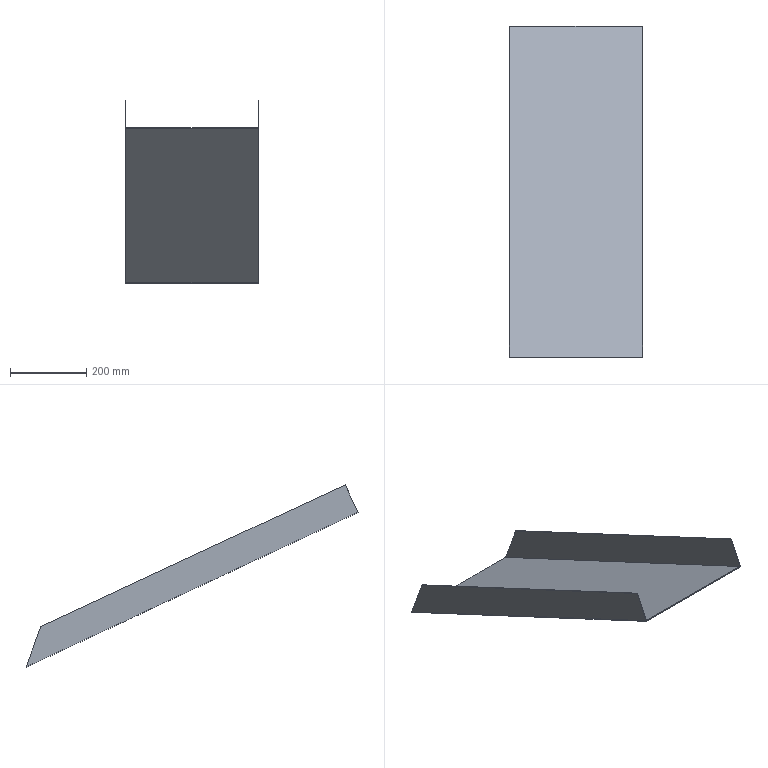Part | NX | features solid 2 | 1 solid | 10 faces | box 350 x 870.242 x 478.305 mm | volume 958236 mm3 | plane 10
STEP:
#1=CARTESIAN_POINT('',(20.,289.829,-157.495));
#2=VERTEX_POINT('',#1);
#3=CARTESIAN_POINT('',(22.,289.829,-157.495));
#4=VERTEX_POINT('',#3);
#5=CARTESIAN_POINT('',(1210.,289.829,-157.495));
#6=DIRECTION('',(-1.,0.,0.));
#7=VECTOR('',#6,1000.);
#8=LINE('',#5,#7);
#9=EDGE_CURVE('',#2,#4,#8,.F.);
#10=ORIENTED_EDGE('',*,*,#9,.F.);
#11=CARTESIAN_POINT('',(20.,256.02,-230.));
#12=VERTEX_POINT('',#11);
#13=CARTESIAN_POINT('',(20.,289.829,-157.495));
#14=DIRECTION('',(0.,-0.4226,-0.9063));
#15=VECTOR('',#14,1000.);
#16=LINE('',#13,#15);
#17=EDGE_CURVE('',#2,#12,#16,.T.);
#18=ORIENTED_EDGE('',*,*,#17,.T.);
#19=CARTESIAN_POINT('',(370.,256.02,-230.));
#20=VERTEX_POINT('',#19);
#21=CARTESIAN_POINT('',(1210.,256.02,-230.));
#22=DIRECTION('',(-1.,0.,0.));
#23=VECTOR('',#22,1000.);
#24=LINE('',#21,#23);
#25=EDGE_CURVE('',#12,#20,#24,.F.);
#26=ORIENTED_EDGE('',*,*,#25,.T.);
#27=CARTESIAN_POINT('',(370.,289.829,-157.495));
#28=VERTEX_POINT('',#27);
#29=CARTESIAN_POINT('',(370.,289.829,-157.495));
#30=DIRECTION('',(0.,-0.4226,-0.9063));
#31=VECTOR('',#30,1000.);
#32=LINE('',#29,#31);
#33=EDGE_CURVE('',#28,#20,#32,.T.);
#34=ORIENTED_EDGE('',*,*,#33,.F.);
#35=CARTESIAN_POINT('',(368.,289.829,-157.495));
#36=VERTEX_POINT('',#35);
#37=CARTESIAN_POINT('',(1210.,289.829,-157.495));
#38=DIRECTION('',(-1.,0.,0.));
#39=VECTOR('',#38,1000.);
#40=LINE('',#37,#39);
#41=EDGE_CURVE('',#36,#28,#40,.F.);
#42=ORIENTED_EDGE('',*,*,#41,.F.);
#43=CARTESIAN_POINT('',(368.,256.865,-228.187));
#44=VERTEX_POINT('',#43);
#45=CARTESIAN_POINT('',(368.,289.829,-157.495));
#46=DIRECTION('',(0.,-0.4226,-0.9063));
#47=VECTOR('',#46,1000.);
#48=LINE('',#45,#47);
#49=EDGE_CURVE('',#36,#44,#48,.T.);
#50=ORIENTED_EDGE('',*,*,#49,.T.);
#51=CARTESIAN_POINT('',(22.,256.865,-228.187));
#52=VERTEX_POINT('',#51);
#53=CARTESIAN_POINT('',(10.,256.865,-228.187));
#54=DIRECTION('',(-1.,0.,0.));
#55=VECTOR('',#54,1000.);
#56=LINE('',#53,#55);
#57=EDGE_CURVE('',#52,#44,#56,.F.);
#58=ORIENTED_EDGE('',*,*,#57,.F.);
#59=CARTESIAN_POINT('',(22.,289.829,-157.495));
#60=DIRECTION('',(0.,-0.4226,-0.9063));
#61=VECTOR('',#60,1000.);
#62=LINE('',#59,#61);
#63=EDGE_CURVE('',#4,#52,#62,.T.);
#64=ORIENTED_EDGE('',*,*,#63,.F.);
#65=EDGE_LOOP('',(#10,#18,#26,#34,#42,#50,#58,#64));
#66=FACE_BOUND('',#65,.T.);
#67=CARTESIAN_POINT('',(1210.,289.829,-157.495));
#68=DIRECTION('',(0.,-0.9063,0.4226));
#69=DIRECTION('',(0.,-0.4226,-0.9063));
#70=AXIS2_PLACEMENT_3D('',#67,#68,#69);
#71=PLANE('',#70);
#72=ADVANCED_FACE('',(#66),#71,.T.);
#73=CARTESIAN_POINT('',(368.,1087.566,-529.486));
#74=VERTEX_POINT('',#73);
#75=CARTESIAN_POINT('',(368.,-205.417,73.442));
#76=DIRECTION('',(0.,-0.9063,0.4226));
#77=VECTOR('',#76,1000.);
#78=LINE('',#75,#77);
#79=EDGE_CURVE('',#36,#74,#78,.F.);
#80=ORIENTED_EDGE('',*,*,#79,.F.);
#81=ORIENTED_EDGE('',*,*,#41,.T.);
#82=CARTESIAN_POINT('',(370.,1087.566,-529.486));
#83=VERTEX_POINT('',#82);
#84=CARTESIAN_POINT('',(370.,-205.417,73.442));
#85=DIRECTION('',(0.,0.9063,-0.4226));
#86=VECTOR('',#85,1000.);
#87=LINE('',#84,#86);
#88=EDGE_CURVE('',#28,#83,#87,.T.);
#89=ORIENTED_EDGE('',*,*,#88,.T.);
#90=CARTESIAN_POINT('',(10.,1087.566,-529.486));
#91=DIRECTION('',(1.,0.,0.));
#92=VECTOR('',#91,1000.);
#93=LINE('',#90,#92);
#94=EDGE_CURVE('',#74,#83,#93,.T.);
#95=ORIENTED_EDGE('',*,*,#94,.F.);
#96=EDGE_LOOP('',(#80,#81,#89,#95));
#97=FACE_BOUND('',#96,.T.);
#98=CARTESIAN_POINT('',(10.,-205.417,73.442));
#99=DIRECTION('',(0.,0.4226,0.9063));
#100=DIRECTION('',(0.,0.9063,-0.4226));
#101=AXIS2_PLACEMENT_3D('',#98,#99,#100);
#102=PLANE('',#101);
#103=ADVANCED_FACE('',(#97),#102,.T.);
#104=ORIENTED_EDGE('',*,*,#88,.F.);
#105=ORIENTED_EDGE('',*,*,#33,.T.);
#106=CARTESIAN_POINT('',(370.,1126.262,-635.8));
#107=VERTEX_POINT('',#106);
#108=CARTESIAN_POINT('',(370.,-239.226,0.9369));
#109=DIRECTION('',(0.,0.9063,-0.4226));
#110=VECTOR('',#109,1000.);
#111=LINE('',#108,#110);
#112=EDGE_CURVE('',#20,#107,#111,.T.);
#113=ORIENTED_EDGE('',*,*,#112,.T.);
#114=CARTESIAN_POINT('',(370.,742.539,418.469));
#115=DIRECTION('',(0.,-0.342,0.9397));
#116=VECTOR('',#115,1000.);
#117=LINE('',#114,#116);
#118=EDGE_CURVE('',#83,#107,#117,.F.);
#119=ORIENTED_EDGE('',*,*,#118,.F.);
#120=EDGE_LOOP('',(#104,#105,#113,#119));
#121=FACE_BOUND('',#120,.T.);
#122=CARTESIAN_POINT('',(370.,-205.417,73.442));
#123=DIRECTION('',(1.,0.,0.));
#124=DIRECTION('',(0.,0.,1.));
#125=AXIS2_PLACEMENT_3D('',#122,#123,#124);
#126=PLANE('',#125);
#127=ADVANCED_FACE('',(#121),#126,.T.);
#128=CARTESIAN_POINT('',(20.,1126.262,-635.8));
#129=VERTEX_POINT('',#128);
#130=CARTESIAN_POINT('',(20.,701.624,-437.789));
#131=DIRECTION('',(0.,-0.9063,0.4226));
#132=VECTOR('',#131,1000.);
#133=LINE('',#130,#132);
#134=EDGE_CURVE('',#129,#12,#133,.T.);
#135=ORIENTED_EDGE('',*,*,#134,.T.);
#136=ORIENTED_EDGE('',*,*,#17,.F.);
#137=CARTESIAN_POINT('',(20.,1087.566,-529.486));
#138=VERTEX_POINT('',#137);
#139=CARTESIAN_POINT('',(20.,735.434,-365.284));
#140=DIRECTION('',(0.,-0.9063,0.4226));
#141=VECTOR('',#140,1000.);
#142=LINE('',#139,#141);
#143=EDGE_CURVE('',#138,#2,#142,.T.);
#144=ORIENTED_EDGE('',*,*,#143,.F.);
#145=CARTESIAN_POINT('',(20.,993.601,-271.319));
#146=DIRECTION('',(0.,0.342,-0.9397));
#147=VECTOR('',#146,1000.);
#148=LINE('',#145,#147);
#149=EDGE_CURVE('',#129,#138,#148,.F.);
#150=ORIENTED_EDGE('',*,*,#149,.F.);
#151=EDGE_LOOP('',(#135,#136,#144,#150));
#152=FACE_BOUND('',#151,.T.);
#153=CARTESIAN_POINT('',(20.,735.434,-365.284));
#154=DIRECTION('',(-1.,0.,0.));
#155=DIRECTION('',(0.,0.,-1.));
#156=AXIS2_PLACEMENT_3D('',#153,#154,#155);
#157=PLANE('',#156);
#158=ADVANCED_FACE('',(#152),#157,.T.);
#159=ORIENTED_EDGE('',*,*,#143,.T.);
#160=ORIENTED_EDGE('',*,*,#9,.T.);
#161=CARTESIAN_POINT('',(22.,1087.566,-529.486));
#162=VERTEX_POINT('',#161);
#163=CARTESIAN_POINT('',(22.,-205.417,73.442));
#164=DIRECTION('',(0.,0.9063,-0.4226));
#165=VECTOR('',#164,1000.);
#166=LINE('',#163,#165);
#167=EDGE_CURVE('',#162,#4,#166,.F.);
#168=ORIENTED_EDGE('',*,*,#167,.F.);
#169=CARTESIAN_POINT('',(22.,1087.566,-529.486));
#170=DIRECTION('',(-1.,0.,0.));
#171=VECTOR('',#170,1000.);
#172=LINE('',#169,#171);
#173=EDGE_CURVE('',#138,#162,#172,.F.);
#174=ORIENTED_EDGE('',*,*,#173,.F.);
#175=EDGE_LOOP('',(#159,#160,#168,#174));
#176=FACE_BOUND('',#175,.T.);
#177=CARTESIAN_POINT('',(10.,-205.417,73.442));
#178=DIRECTION('',(0.,0.4226,0.9063));
#179=DIRECTION('',(0.,0.9063,-0.4226));
#180=AXIS2_PLACEMENT_3D('',#177,#178,#179);
#181=PLANE('',#180);
#182=ADVANCED_FACE('',(#176),#181,.T.);
#183=ORIENTED_EDGE('',*,*,#112,.F.);
#184=ORIENTED_EDGE('',*,*,#25,.F.);
#185=ORIENTED_EDGE('',*,*,#134,.F.);
#186=CARTESIAN_POINT('',(10.,1126.262,-635.8));
#187=DIRECTION('',(1.,0.,0.));
#188=VECTOR('',#187,1000.);
#189=LINE('',#186,#188);
#190=EDGE_CURVE('',#107,#129,#189,.F.);
#191=ORIENTED_EDGE('',*,*,#190,.F.);
#192=EDGE_LOOP('',(#183,#184,#185,#191));
#193=FACE_BOUND('',#192,.T.);
#194=CARTESIAN_POINT('',(10.,-239.226,0.9369));
#195=DIRECTION('',(0.,0.4226,0.9063));
#196=DIRECTION('',(0.,0.9063,-0.4226));
#197=AXIS2_PLACEMENT_3D('',#194,#195,#196);
#198=PLANE('',#197);
#199=ADVANCED_FACE('',(#193),#198,.F.);
#200=CARTESIAN_POINT('',(368.,1125.294,-633.143));
#201=VERTEX_POINT('',#200);
#202=CARTESIAN_POINT('',(368.,-238.381,2.75));
#203=DIRECTION('',(0.,-0.9063,0.4226));
#204=VECTOR('',#203,1000.);
#205=LINE('',#202,#204);
#206=EDGE_CURVE('',#44,#201,#205,.F.);
#207=ORIENTED_EDGE('',*,*,#206,.F.);
#208=ORIENTED_EDGE('',*,*,#49,.F.);
#209=ORIENTED_EDGE('',*,*,#79,.T.);
#210=CARTESIAN_POINT('',(368.,1126.262,-635.8));
#211=DIRECTION('',(0.,0.342,-0.9397));
#212=VECTOR('',#211,1000.);
#213=LINE('',#210,#212);
#214=EDGE_CURVE('',#201,#74,#213,.F.);
#215=ORIENTED_EDGE('',*,*,#214,.F.);
#216=EDGE_LOOP('',(#207,#208,#209,#215));
#217=FACE_BOUND('',#216,.T.);
#218=CARTESIAN_POINT('',(368.,-205.417,73.442));
#219=DIRECTION('',(1.,0.,0.));
#220=DIRECTION('',(0.,0.,1.));
#221=AXIS2_PLACEMENT_3D('',#218,#219,#220);
#222=PLANE('',#221);
#223=ADVANCED_FACE('',(#217),#222,.F.);
#224=ORIENTED_EDGE('',*,*,#167,.T.);
#225=ORIENTED_EDGE('',*,*,#63,.T.);
#226=CARTESIAN_POINT('',(22.,1125.294,-633.143));
#227=VERTEX_POINT('',#226);
#228=CARTESIAN_POINT('',(22.,-238.381,2.75));
#229=DIRECTION('',(0.,0.9063,-0.4226));
#230=VECTOR('',#229,1000.);
#231=LINE('',#228,#230);
#232=EDGE_CURVE('',#227,#52,#231,.F.);
#233=ORIENTED_EDGE('',*,*,#232,.F.);
#234=CARTESIAN_POINT('',(22.,1126.262,-635.8));
#235=DIRECTION('',(0.,-0.342,0.9397));
#236=VECTOR('',#235,1000.);
#237=LINE('',#234,#236);
#238=EDGE_CURVE('',#162,#227,#237,.F.);
#239=ORIENTED_EDGE('',*,*,#238,.F.);
#240=EDGE_LOOP('',(#224,#225,#233,#239));
#241=FACE_BOUND('',#240,.T.);
#242=CARTESIAN_POINT('',(22.,735.434,-365.284));
#243=DIRECTION('',(-1.,0.,0.));
#244=DIRECTION('',(0.,0.,-1.));
#245=AXIS2_PLACEMENT_3D('',#242,#243,#244);
#246=PLANE('',#245);
#247=ADVANCED_FACE('',(#241),#246,.F.);
#248=ORIENTED_EDGE('',*,*,#232,.T.);
#249=ORIENTED_EDGE('',*,*,#57,.T.);
#250=ORIENTED_EDGE('',*,*,#206,.T.);
#251=CARTESIAN_POINT('',(10.,1125.294,-633.143));
#252=DIRECTION('',(1.,0.,0.));
#253=VECTOR('',#252,1000.);
#254=LINE('',#251,#253);
#255=EDGE_CURVE('',#227,#201,#254,.T.);
#256=ORIENTED_EDGE('',*,*,#255,.F.);
#257=EDGE_LOOP('',(#248,#249,#250,#256));
#258=FACE_BOUND('',#257,.T.);
#259=CARTESIAN_POINT('',(10.,-238.381,2.75));
#260=DIRECTION('',(0.,0.4226,0.9063));
#261=DIRECTION('',(0.,0.9063,-0.4226));
#262=AXIS2_PLACEMENT_3D('',#259,#260,#261);
#263=PLANE('',#262);
#264=ADVANCED_FACE('',(#258),#263,.T.);
#265=ORIENTED_EDGE('',*,*,#238,.T.);
#266=ORIENTED_EDGE('',*,*,#255,.T.);
#267=ORIENTED_EDGE('',*,*,#214,.T.);
#268=ORIENTED_EDGE('',*,*,#94,.T.);
#269=ORIENTED_EDGE('',*,*,#118,.T.);
#270=ORIENTED_EDGE('',*,*,#190,.T.);
#271=ORIENTED_EDGE('',*,*,#149,.T.);
#272=ORIENTED_EDGE('',*,*,#173,.T.);
#273=EDGE_LOOP('',(#265,#266,#267,#268,#269,#270,#271,#272));
#274=FACE_BOUND('',#273,.T.);
#275=CARTESIAN_POINT('',(10.,1126.262,-635.8));
#276=DIRECTION('',(0.,-0.9397,-0.342));
#277=DIRECTION('',(0.,0.342,-0.9397));
#278=AXIS2_PLACEMENT_3D('',#275,#276,#277);
#279=PLANE('',#278);
#280=ADVANCED_FACE('',(#274),#279,.F.);
#281=CLOSED_SHELL('',(#72,#103,#127,#158,#182,#199,#223,#247,#264,#280));
#282=MANIFOLD_SOLID_BREP('',#281);
#283=(LENGTH_UNIT()NAMED_UNIT(*)SI_UNIT(.MILLI.,.METRE.));
#284=UNCERTAINTY_MEASURE_WITH_UNIT(LENGTH_MEASURE(0.00001),#283,'','');
#285=(NAMED_UNIT(*)PLANE_ANGLE_UNIT()SI_UNIT($,.RADIAN.));
#286=(NAMED_UNIT(*)SI_UNIT($,.STERADIAN.)SOLID_ANGLE_UNIT());
#287=(GEOMETRIC_REPRESENTATION_CONTEXT(3)GLOBAL_UNCERTAINTY_ASSIGNED_CONTEXT((#284))GLOBAL_UNIT_ASSIGNED_CONTEXT((#283,#285,#286))REPRESENTATION_CONTEXT('',''));
#288=ADVANCED_BREP_SHAPE_REPRESENTATION('',(#282),#287);